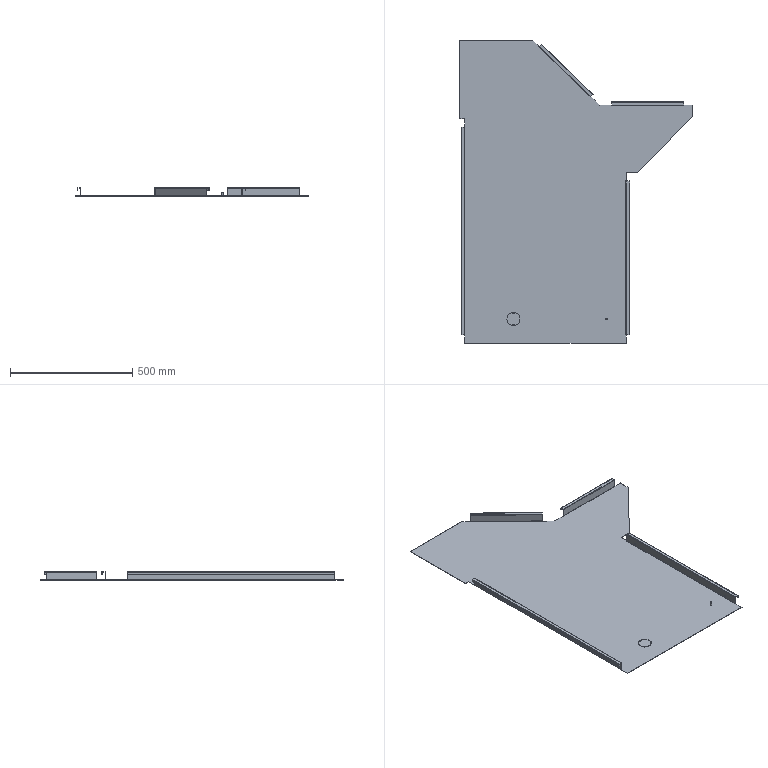Part | SolidWorks | features EdgeFlange 3, ICE 2, FlatPattern 1, FormToolInstance 1, SMBaseFlange 1, SheetMetal 1 | 1 solid | 146 faces | box 952.629 x 1240 x 35 mm | volume 1386350 mm3 | plane 104 | cylinder 38 | torus 4 | commonest cylinder face diameters 0.2 x12 3.2 x12 7 x4 50 x3 53 x3 6 x2